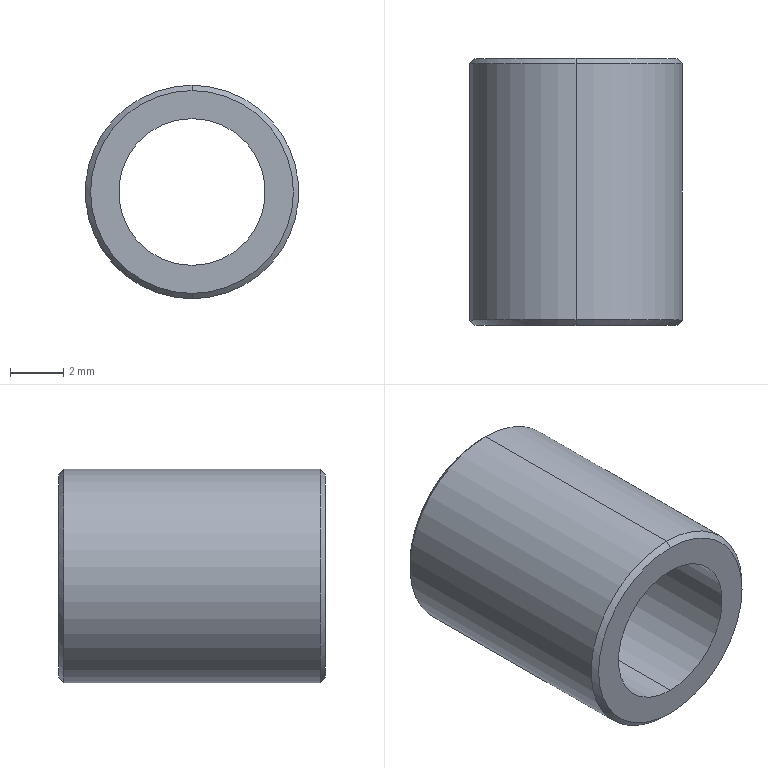Part | SolidWorks | features Chamfer 1, Extrusion 1 | 1 solid | 10 faces | box 8 x 10 x 8 mm | volume 264.083 mm3 | cone 4 | cylinder 4 | plane 2 | commonest cylinder face diameters 5.5 x2 8 x2
STEP:
#1=CARTESIAN_POINT('',(0.,10.,3.8));
#2=VERTEX_POINT('',#1);
#3=CARTESIAN_POINT('',(0.,10.,-3.8));
#4=VERTEX_POINT('',#3);
#5=CARTESIAN_POINT('',(0.,10.,0.));
#6=DIRECTION('',(0.,1.,0.));
#7=DIRECTION('',(0.,0.,1.));
#8=AXIS2_PLACEMENT_3D('',#5,#6,#7);
#9=CIRCLE('',#8,3.8);
#10=EDGE_CURVE('',#2,#4,#9,.T.);
#11=ORIENTED_EDGE('',*,*,#10,.F.);
#12=CARTESIAN_POINT('',(0.,9.8,4.));
#13=VERTEX_POINT('',#12);
#14=CARTESIAN_POINT('',(0.,10.,3.8));
#15=DIRECTION('',(0.,-0.7071,0.7071));
#16=VECTOR('',#15,1000.);
#17=LINE('',#14,#16);
#18=EDGE_CURVE('',#2,#13,#17,.T.);
#19=ORIENTED_EDGE('',*,*,#18,.T.);
#20=CARTESIAN_POINT('',(0.,9.8,-4.));
#21=VERTEX_POINT('',#20);
#22=CARTESIAN_POINT('',(0.,9.8,0.));
#23=DIRECTION('',(0.,-1.,0.));
#24=DIRECTION('',(0.,0.,1.));
#25=AXIS2_PLACEMENT_3D('',#22,#23,#24);
#26=CIRCLE('',#25,4.);
#27=EDGE_CURVE('',#21,#13,#26,.T.);
#28=ORIENTED_EDGE('',*,*,#27,.F.);
#29=CARTESIAN_POINT('',(0.,10.,-3.8));
#30=DIRECTION('',(0.,-0.7071,-0.7071));
#31=VECTOR('',#30,1000.);
#32=LINE('',#29,#31);
#33=EDGE_CURVE('',#4,#21,#32,.T.);
#34=ORIENTED_EDGE('',*,*,#33,.F.);
#35=EDGE_LOOP('',(#11,#19,#28,#34));
#36=FACE_OUTER_BOUND('',#35,.T.);
#37=CARTESIAN_POINT('',(0.,10.,0.));
#38=DIRECTION('',(0.,-1.,0.));
#39=DIRECTION('',(0.,0.,-1.));
#40=AXIS2_PLACEMENT_3D('',#37,#38,#39);
#41=CONICAL_SURFACE('',#40,3.8,0.7854);
#42=ADVANCED_FACE('',(#36),#41,.T.);
#43=CARTESIAN_POINT('',(0.,0.,-3.8));
#44=VERTEX_POINT('',#43);
#45=CARTESIAN_POINT('',(0.,0.,3.8));
#46=VERTEX_POINT('',#45);
#47=CARTESIAN_POINT('',(0.,0.,0.));
#48=DIRECTION('',(0.,-1.,0.));
#49=DIRECTION('',(0.,0.,1.));
#50=AXIS2_PLACEMENT_3D('',#47,#48,#49);
#51=CIRCLE('',#50,3.8);
#52=EDGE_CURVE('',#44,#46,#51,.T.);
#53=ORIENTED_EDGE('',*,*,#52,.F.);
#54=CARTESIAN_POINT('',(0.,0.2,-4.));
#55=VERTEX_POINT('',#54);
#56=CARTESIAN_POINT('',(0.,0.2,-4.));
#57=DIRECTION('',(0.,0.7071,-0.7071));
#58=VECTOR('',#57,1000.);
#59=LINE('',#56,#58);
#60=EDGE_CURVE('',#44,#55,#59,.T.);
#61=ORIENTED_EDGE('',*,*,#60,.T.);
#62=CARTESIAN_POINT('',(0.,0.2,4.));
#63=VERTEX_POINT('',#62);
#64=CARTESIAN_POINT('',(0.,0.2,0.));
#65=DIRECTION('',(0.,1.,0.));
#66=DIRECTION('',(0.,0.,1.));
#67=AXIS2_PLACEMENT_3D('',#64,#65,#66);
#68=CIRCLE('',#67,4.);
#69=EDGE_CURVE('',#63,#55,#68,.T.);
#70=ORIENTED_EDGE('',*,*,#69,.F.);
#71=CARTESIAN_POINT('',(0.,0.2,4.));
#72=DIRECTION('',(0.,0.7071,0.7071));
#73=VECTOR('',#72,1000.);
#74=LINE('',#71,#73);
#75=EDGE_CURVE('',#46,#63,#74,.T.);
#76=ORIENTED_EDGE('',*,*,#75,.F.);
#77=EDGE_LOOP('',(#53,#61,#70,#76));
#78=FACE_OUTER_BOUND('',#77,.T.);
#79=CARTESIAN_POINT('',(0.,0.2,0.));
#80=DIRECTION('',(0.,1.,0.));
#81=DIRECTION('',(0.,0.,1.));
#82=AXIS2_PLACEMENT_3D('',#79,#80,#81);
#83=CONICAL_SURFACE('',#82,4.,0.7854);
#84=ADVANCED_FACE('',(#78),#83,.T.);
#85=CARTESIAN_POINT('',(0.,10.,-2.75));
#86=VERTEX_POINT('',#85);
#87=CARTESIAN_POINT('',(0.,10.,2.75));
#88=VERTEX_POINT('',#87);
#89=CARTESIAN_POINT('',(0.,10.,0.));
#90=DIRECTION('',(0.,1.,0.));
#91=DIRECTION('',(0.,0.,1.));
#92=AXIS2_PLACEMENT_3D('',#89,#90,#91);
#93=CIRCLE('',#92,2.75);
#94=EDGE_CURVE('',#86,#88,#93,.T.);
#95=ORIENTED_EDGE('',*,*,#94,.T.);
#96=CARTESIAN_POINT('',(0.,0.,2.75));
#97=VERTEX_POINT('',#96);
#98=CARTESIAN_POINT('',(0.,10.,2.75));
#99=DIRECTION('',(0.,-1.,0.));
#100=VECTOR('',#99,1000.);
#101=LINE('',#98,#100);
#102=EDGE_CURVE('',#88,#97,#101,.T.);
#103=ORIENTED_EDGE('',*,*,#102,.T.);
#104=CARTESIAN_POINT('',(0.,0.,-2.75));
#105=VERTEX_POINT('',#104);
#106=CARTESIAN_POINT('',(0.,0.,0.));
#107=DIRECTION('',(0.,1.,0.));
#108=DIRECTION('',(0.,0.,1.));
#109=AXIS2_PLACEMENT_3D('',#106,#107,#108);
#110=CIRCLE('',#109,2.75);
#111=EDGE_CURVE('',#105,#97,#110,.T.);
#112=ORIENTED_EDGE('',*,*,#111,.F.);
#113=CARTESIAN_POINT('',(0.,10.,-2.75));
#114=DIRECTION('',(0.,-1.,0.));
#115=VECTOR('',#114,1000.);
#116=LINE('',#113,#115);
#117=EDGE_CURVE('',#86,#105,#116,.T.);
#118=ORIENTED_EDGE('',*,*,#117,.F.);
#119=EDGE_LOOP('',(#95,#103,#112,#118));
#120=FACE_OUTER_BOUND('',#119,.T.);
#121=CARTESIAN_POINT('',(0.,10.,0.));
#122=DIRECTION('',(0.,-1.,0.));
#123=DIRECTION('',(0.,0.,-1.));
#124=AXIS2_PLACEMENT_3D('',#121,#122,#123);
#125=CYLINDRICAL_SURFACE('',#124,2.75);
#126=ADVANCED_FACE('',(#120),#125,.F.);
#127=ORIENTED_EDGE('',*,*,#27,.T.);
#128=CARTESIAN_POINT('',(0.,10.,4.));
#129=DIRECTION('',(0.,-1.,0.));
#130=VECTOR('',#129,1000.);
#131=LINE('',#128,#130);
#132=EDGE_CURVE('',#13,#63,#131,.T.);
#133=ORIENTED_EDGE('',*,*,#132,.T.);
#134=ORIENTED_EDGE('',*,*,#69,.T.);
#135=CARTESIAN_POINT('',(0.,10.,-4.));
#136=DIRECTION('',(0.,-1.,0.));
#137=VECTOR('',#136,1000.);
#138=LINE('',#135,#137);
#139=EDGE_CURVE('',#21,#55,#138,.T.);
#140=ORIENTED_EDGE('',*,*,#139,.F.);
#141=EDGE_LOOP('',(#127,#133,#134,#140));
#142=FACE_OUTER_BOUND('',#141,.T.);
#143=CARTESIAN_POINT('',(0.,10.,0.));
#144=DIRECTION('',(0.,-1.,0.));
#145=DIRECTION('',(0.,0.,-1.));
#146=AXIS2_PLACEMENT_3D('',#143,#144,#145);
#147=CYLINDRICAL_SURFACE('',#146,4.);
#148=ADVANCED_FACE('',(#142),#147,.T.);
#149=CARTESIAN_POINT('',(0.,10.,0.));
#150=DIRECTION('',(0.,1.,0.));
#151=DIRECTION('',(0.,0.,1.));
#152=AXIS2_PLACEMENT_3D('',#149,#150,#151);
#153=CIRCLE('',#152,3.8);
#154=EDGE_CURVE('',#4,#2,#153,.T.);
#155=ORIENTED_EDGE('',*,*,#154,.T.);
#156=ORIENTED_EDGE('',*,*,#10,.T.);
#157=EDGE_LOOP('',(#155,#156));
#158=FACE_OUTER_BOUND('',#157,.T.);
#159=ORIENTED_EDGE('',*,*,#94,.F.);
#160=CARTESIAN_POINT('',(0.,10.,0.));
#161=DIRECTION('',(0.,1.,0.));
#162=DIRECTION('',(0.,0.,1.));
#163=AXIS2_PLACEMENT_3D('',#160,#161,#162);
#164=CIRCLE('',#163,2.75);
#165=EDGE_CURVE('',#88,#86,#164,.T.);
#166=ORIENTED_EDGE('',*,*,#165,.F.);
#167=EDGE_LOOP('',(#159,#166));
#168=FACE_BOUND('',#167,.T.);
#169=CARTESIAN_POINT('',(0.,10.,0.));
#170=DIRECTION('',(0.,1.,0.));
#171=DIRECTION('',(0.,0.,1.));
#172=AXIS2_PLACEMENT_3D('',#169,#170,#171);
#173=PLANE('',#172);
#174=ADVANCED_FACE('',(#158,#168),#173,.T.);
#175=CARTESIAN_POINT('',(0.,0.,0.));
#176=DIRECTION('',(0.,-1.,0.));
#177=DIRECTION('',(0.,0.,1.));
#178=AXIS2_PLACEMENT_3D('',#175,#176,#177);
#179=CIRCLE('',#178,3.8);
#180=EDGE_CURVE('',#46,#44,#179,.T.);
#181=ORIENTED_EDGE('',*,*,#180,.T.);
#182=ORIENTED_EDGE('',*,*,#52,.T.);
#183=EDGE_LOOP('',(#181,#182));
#184=FACE_OUTER_BOUND('',#183,.T.);
#185=ORIENTED_EDGE('',*,*,#111,.T.);
#186=CARTESIAN_POINT('',(0.,0.,0.));
#187=DIRECTION('',(0.,1.,0.));
#188=DIRECTION('',(0.,0.,1.));
#189=AXIS2_PLACEMENT_3D('',#186,#187,#188);
#190=CIRCLE('',#189,2.75);
#191=EDGE_CURVE('',#97,#105,#190,.T.);
#192=ORIENTED_EDGE('',*,*,#191,.T.);
#193=EDGE_LOOP('',(#185,#192));
#194=FACE_BOUND('',#193,.T.);
#195=CARTESIAN_POINT('',(0.,0.,0.));
#196=DIRECTION('',(0.,1.,0.));
#197=DIRECTION('',(0.,0.,1.));
#198=AXIS2_PLACEMENT_3D('',#195,#196,#197);
#199=PLANE('',#198);
#200=ADVANCED_FACE('',(#184,#194),#199,.F.);
#201=ORIENTED_EDGE('',*,*,#132,.F.);
#202=CARTESIAN_POINT('',(0.,9.8,0.));
#203=DIRECTION('',(0.,-1.,0.));
#204=DIRECTION('',(0.,0.,1.));
#205=AXIS2_PLACEMENT_3D('',#202,#203,#204);
#206=CIRCLE('',#205,4.);
#207=EDGE_CURVE('',#13,#21,#206,.T.);
#208=ORIENTED_EDGE('',*,*,#207,.T.);
#209=ORIENTED_EDGE('',*,*,#139,.T.);
#210=CARTESIAN_POINT('',(0.,0.2,0.));
#211=DIRECTION('',(0.,1.,0.));
#212=DIRECTION('',(0.,0.,1.));
#213=AXIS2_PLACEMENT_3D('',#210,#211,#212);
#214=CIRCLE('',#213,4.);
#215=EDGE_CURVE('',#55,#63,#214,.T.);
#216=ORIENTED_EDGE('',*,*,#215,.T.);
#217=EDGE_LOOP('',(#201,#208,#209,#216));
#218=FACE_OUTER_BOUND('',#217,.T.);
#219=CARTESIAN_POINT('',(0.,10.,0.));
#220=DIRECTION('',(0.,-1.,0.));
#221=DIRECTION('',(0.,0.,-1.));
#222=AXIS2_PLACEMENT_3D('',#219,#220,#221);
#223=CYLINDRICAL_SURFACE('',#222,4.);
#224=ADVANCED_FACE('',(#218),#223,.T.);
#225=ORIENTED_EDGE('',*,*,#102,.F.);
#226=ORIENTED_EDGE('',*,*,#165,.T.);
#227=ORIENTED_EDGE('',*,*,#117,.T.);
#228=ORIENTED_EDGE('',*,*,#191,.F.);
#229=EDGE_LOOP('',(#225,#226,#227,#228));
#230=FACE_OUTER_BOUND('',#229,.T.);
#231=CARTESIAN_POINT('',(0.,10.,0.));
#232=DIRECTION('',(0.,-1.,0.));
#233=DIRECTION('',(0.,0.,-1.));
#234=AXIS2_PLACEMENT_3D('',#231,#232,#233);
#235=CYLINDRICAL_SURFACE('',#234,2.75);
#236=ADVANCED_FACE('',(#230),#235,.F.);
#237=ORIENTED_EDGE('',*,*,#60,.F.);
#238=ORIENTED_EDGE('',*,*,#180,.F.);
#239=ORIENTED_EDGE('',*,*,#75,.T.);
#240=ORIENTED_EDGE('',*,*,#215,.F.);
#241=EDGE_LOOP('',(#237,#238,#239,#240));
#242=FACE_OUTER_BOUND('',#241,.T.);
#243=CARTESIAN_POINT('',(0.,0.2,0.));
#244=DIRECTION('',(0.,1.,0.));
#245=DIRECTION('',(0.,0.,1.));
#246=AXIS2_PLACEMENT_3D('',#243,#244,#245);
#247=CONICAL_SURFACE('',#246,4.,0.7854);
#248=ADVANCED_FACE('',(#242),#247,.T.);
#249=ORIENTED_EDGE('',*,*,#18,.F.);
#250=ORIENTED_EDGE('',*,*,#154,.F.);
#251=ORIENTED_EDGE('',*,*,#33,.T.);
#252=ORIENTED_EDGE('',*,*,#207,.F.);
#253=EDGE_LOOP('',(#249,#250,#251,#252));
#254=FACE_OUTER_BOUND('',#253,.T.);
#255=CARTESIAN_POINT('',(0.,10.,0.));
#256=DIRECTION('',(0.,-1.,0.));
#257=DIRECTION('',(0.,0.,-1.));
#258=AXIS2_PLACEMENT_3D('',#255,#256,#257);
#259=CONICAL_SURFACE('',#258,3.8,0.7854);
#260=ADVANCED_FACE('',(#254),#259,.T.);
#261=CLOSED_SHELL('',(#42,#84,#126,#148,#174,#200,#224,#236,#248,#260));
#262=MANIFOLD_SOLID_BREP('',#261);
#263=CARTESIAN_POINT('',(0.,0.,0.));
#264=DIRECTION('',(0.,0.,1.));
#265=DIRECTION('',(1.,0.,0.));
#266=AXIS2_PLACEMENT_3D('',#263,#264,#265);
#267=(LENGTH_UNIT()NAMED_UNIT(*)SI_UNIT(.MILLI.,.METRE.));
#268=UNCERTAINTY_MEASURE_WITH_UNIT(LENGTH_MEASURE(0.00001),#267,'','');
#269=(NAMED_UNIT(*)PLANE_ANGLE_UNIT()SI_UNIT($,.RADIAN.));
#270=(NAMED_UNIT(*)SI_UNIT($,.STERADIAN.)SOLID_ANGLE_UNIT());
#271=(GEOMETRIC_REPRESENTATION_CONTEXT(3)GLOBAL_UNCERTAINTY_ASSIGNED_CONTEXT((#268))GLOBAL_UNIT_ASSIGNED_CONTEXT((#267,#269,#270))REPRESENTATION_CONTEXT('',''));
#272=ADVANCED_BREP_SHAPE_REPRESENTATION('',(#262,#266),#271);